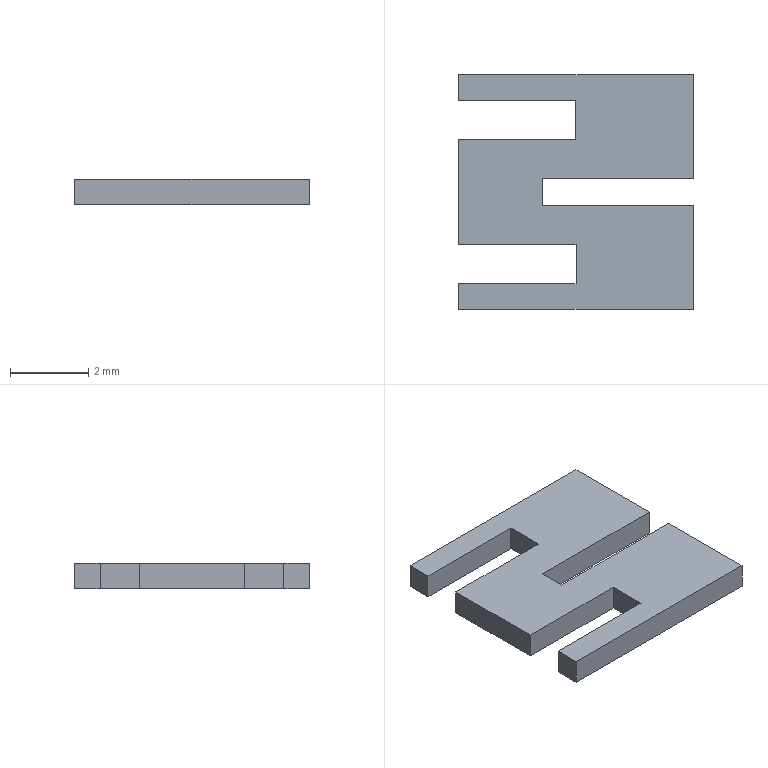Part | STEP file | RJ-USIO-V1_2-220411_176 | 1 solid | 18 faces | box 6 x 6 x 0.65 mm | volume 17.741 mm3 | plane 18
STEP:
#1=CARTESIAN_POINT('',(0.,0.,0.));
#2=DIRECTION('',(0.,0.,1.));
#3=DIRECTION('',(1.,0.,0.));
#4=AXIS2_PLACEMENT_3D('',#1,#2,#3);
#5=CARTESIAN_POINT('',(100.284,60.75,4.15));
#6=VERTEX_POINT('',#5);
#7=CARTESIAN_POINT('',(100.284,60.75,4.8));
#8=VERTEX_POINT('',#7);
#9=CARTESIAN_POINT('',(100.284,60.75,4.15));
#10=DIRECTION('',(0.,0.,1.));
#11=VECTOR('',#10,1.);
#12=LINE('',#9,#11);
#13=CARTESIAN_POINT('',(100.284,60.4,4.475));
#14=DIRECTION('',(1.,0.000000012,0.));
#15=DIRECTION('',(0.,0.,1.));
#16=AXIS2_PLACEMENT_3D('',#13,#14,#15);
#17=PLANE('',#16);
#18=CARTESIAN_POINT('',(-0.325,-0.35));
#19=DIRECTION('',(1.,0.));
#20=VECTOR('',#19,1.);
#21=LINE('',#18,#20);
#22=(GEOMETRIC_REPRESENTATION_CONTEXT(2)PARAMETRIC_REPRESENTATION_CONTEXT()REPRESENTATION_CONTEXT('',''));
#23=DEFINITIONAL_REPRESENTATION('',(#21),#22);
#24=PCURVE('',#17,#23);
#25=CARTESIAN_POINT('',(102.217,60.75,4.475));
#26=DIRECTION('',(0.000000012,-1.,0.));
#27=DIRECTION('',(0.,0.,-1.));
#28=AXIS2_PLACEMENT_3D('',#25,#26,#27);
#29=PLANE('',#28);
#30=CARTESIAN_POINT('',(0.325,-1.933));
#31=DIRECTION('',(-1.,0.));
#32=VECTOR('',#31,1.);
#33=LINE('',#30,#32);
#34=(GEOMETRIC_REPRESENTATION_CONTEXT(2)PARAMETRIC_REPRESENTATION_CONTEXT()REPRESENTATION_CONTEXT('',''));
#35=DEFINITIONAL_REPRESENTATION('',(#33),#34);
#36=PCURVE('',#29,#35);
#37=SURFACE_CURVE('',#12,(#24,#36),.PCURVE_S1.);
#38=EDGE_CURVE('',#6,#8,#37,.T.);
#39=ORIENTED_EDGE('',*,*,#38,.F.);
#40=CARTESIAN_POINT('',(100.284,60.05,4.15));
#41=VERTEX_POINT('',#40);
#42=CARTESIAN_POINT('',(100.284,60.05,4.15));
#43=DIRECTION('',(-0.000000012,1.,0.));
#44=VECTOR('',#43,1.);
#45=LINE('',#42,#44);
#46=CARTESIAN_POINT('',(-0.325,0.35));
#47=DIRECTION('',(0.,-1.));
#48=VECTOR('',#47,1.);
#49=LINE('',#46,#48);
#50=(GEOMETRIC_REPRESENTATION_CONTEXT(2)PARAMETRIC_REPRESENTATION_CONTEXT()REPRESENTATION_CONTEXT('',''));
#51=DEFINITIONAL_REPRESENTATION('',(#49),#50);
#52=PCURVE('',#17,#51);
#53=CARTESIAN_POINT('',(101.15,60.4,4.15));
#54=DIRECTION('',(0.,0.,1.));
#55=DIRECTION('',(-0.000000012,1.,0.));
#56=AXIS2_PLACEMENT_3D('',#53,#54,#55);
#57=PLANE('',#56);
#58=CARTESIAN_POINT('',(-0.35,0.8663));
#59=DIRECTION('',(1.,0.));
#60=VECTOR('',#59,1.);
#61=LINE('',#58,#60);
#62=(GEOMETRIC_REPRESENTATION_CONTEXT(2)PARAMETRIC_REPRESENTATION_CONTEXT()REPRESENTATION_CONTEXT('',''));
#63=DEFINITIONAL_REPRESENTATION('',(#61),#62);
#64=PCURVE('',#57,#63);
#65=SURFACE_CURVE('',#45,(#52,#64),.PCURVE_S1.);
#66=EDGE_CURVE('',#41,#6,#65,.T.);
#67=ORIENTED_EDGE('',*,*,#66,.F.);
#68=CARTESIAN_POINT('',(100.284,60.05,4.8));
#69=VERTEX_POINT('',#68);
#70=CARTESIAN_POINT('',(100.284,60.05,4.15));
#71=DIRECTION('',(0.,0.,1.));
#72=VECTOR('',#71,1.);
#73=LINE('',#70,#72);
#74=CARTESIAN_POINT('',(-0.325,0.35));
#75=DIRECTION('',(1.,0.));
#76=VECTOR('',#75,1.);
#77=LINE('',#74,#76);
#78=(GEOMETRIC_REPRESENTATION_CONTEXT(2)PARAMETRIC_REPRESENTATION_CONTEXT()REPRESENTATION_CONTEXT('',''));
#79=DEFINITIONAL_REPRESENTATION('',(#77),#78);
#80=PCURVE('',#17,#79);
#81=CARTESIAN_POINT('',(102.217,60.05,4.475));
#82=DIRECTION('',(0.000000012,-1.,0.));
#83=DIRECTION('',(-1.,-0.000000012,0.));
#84=AXIS2_PLACEMENT_3D('',#81,#82,#83);
#85=PLANE('',#84);
#86=CARTESIAN_POINT('',(1.933,0.325));
#87=DIRECTION('',(0.,-1.));
#88=VECTOR('',#87,1.);
#89=LINE('',#86,#88);
#90=(GEOMETRIC_REPRESENTATION_CONTEXT(2)PARAMETRIC_REPRESENTATION_CONTEXT()REPRESENTATION_CONTEXT('',''));
#91=DEFINITIONAL_REPRESENTATION('',(#89),#90);
#92=PCURVE('',#85,#91);
#93=SURFACE_CURVE('',#73,(#80,#92),.PCURVE_S1.);
#94=EDGE_CURVE('',#41,#69,#93,.T.);
#95=ORIENTED_EDGE('',*,*,#94,.T.);
#96=CARTESIAN_POINT('',(100.284,60.05,4.8));
#97=DIRECTION('',(-0.000000012,1.,0.));
#98=VECTOR('',#97,1.);
#99=LINE('',#96,#98);
#100=CARTESIAN_POINT('',(0.325,0.35));
#101=DIRECTION('',(0.,-1.));
#102=VECTOR('',#101,1.);
#103=LINE('',#100,#102);
#104=(GEOMETRIC_REPRESENTATION_CONTEXT(2)PARAMETRIC_REPRESENTATION_CONTEXT()REPRESENTATION_CONTEXT('',''));
#105=DEFINITIONAL_REPRESENTATION('',(#103),#104);
#106=PCURVE('',#17,#105);
#107=CARTESIAN_POINT('',(101.15,60.4,4.8));
#108=DIRECTION('',(0.,0.,1.));
#109=DIRECTION('',(-0.000000012,1.,0.));
#110=AXIS2_PLACEMENT_3D('',#107,#108,#109);
#111=PLANE('',#110);
#112=CARTESIAN_POINT('',(-0.35,0.8663));
#113=DIRECTION('',(1.,0.));
#114=VECTOR('',#113,1.);
#115=LINE('',#112,#114);
#116=(GEOMETRIC_REPRESENTATION_CONTEXT(2)PARAMETRIC_REPRESENTATION_CONTEXT()REPRESENTATION_CONTEXT('',''));
#117=DEFINITIONAL_REPRESENTATION('',(#115),#116);
#118=PCURVE('',#111,#117);
#119=SURFACE_CURVE('',#99,(#106,#118),.PCURVE_S1.);
#120=EDGE_CURVE('',#69,#8,#119,.T.);
#121=ORIENTED_EDGE('',*,*,#120,.T.);
#122=EDGE_LOOP('',(#39,#67,#95,#121));
#123=FACE_BOUND('',#122,.F.);
#124=ADVANCED_FACE('',(#123),#17,.T.);
#125=CARTESIAN_POINT('',(104.15,60.75,4.15));
#126=VERTEX_POINT('',#125);
#127=CARTESIAN_POINT('',(104.15,60.75,4.8));
#128=VERTEX_POINT('',#127);
#129=CARTESIAN_POINT('',(104.15,60.75,4.15));
#130=DIRECTION('',(0.,0.,1.));
#131=VECTOR('',#130,1.);
#132=LINE('',#129,#131);
#133=CARTESIAN_POINT('',(0.325,1.933));
#134=DIRECTION('',(-1.,0.));
#135=VECTOR('',#134,1.);
#136=LINE('',#133,#135);
#137=(GEOMETRIC_REPRESENTATION_CONTEXT(2)PARAMETRIC_REPRESENTATION_CONTEXT()REPRESENTATION_CONTEXT('',''));
#138=DEFINITIONAL_REPRESENTATION('',(#136),#137);
#139=PCURVE('',#29,#138);
#140=CARTESIAN_POINT('',(104.15,62.075,4.475));
#141=DIRECTION('',(1.,0.000000012,0.));
#142=DIRECTION('',(0.,0.,1.));
#143=AXIS2_PLACEMENT_3D('',#140,#141,#142);
#144=PLANE('',#143);
#145=CARTESIAN_POINT('',(-0.325,1.325));
#146=DIRECTION('',(1.,0.));
#147=VECTOR('',#146,1.);
#148=LINE('',#145,#147);
#149=(GEOMETRIC_REPRESENTATION_CONTEXT(2)PARAMETRIC_REPRESENTATION_CONTEXT()REPRESENTATION_CONTEXT('',''));
#150=DEFINITIONAL_REPRESENTATION('',(#148),#149);
#151=PCURVE('',#144,#150);
#152=SURFACE_CURVE('',#132,(#139,#151),.PCURVE_S1.);
#153=EDGE_CURVE('',#126,#128,#152,.T.);
#154=ORIENTED_EDGE('',*,*,#153,.F.);
#155=CARTESIAN_POINT('',(100.284,60.75,4.15));
#156=DIRECTION('',(1.,0.000000012,0.));
#157=VECTOR('',#156,1.);
#158=LINE('',#155,#157);
#159=CARTESIAN_POINT('',(0.325,-1.933));
#160=DIRECTION('',(0.,1.));
#161=VECTOR('',#160,1.);
#162=LINE('',#159,#161);
#163=(GEOMETRIC_REPRESENTATION_CONTEXT(2)PARAMETRIC_REPRESENTATION_CONTEXT()REPRESENTATION_CONTEXT('',''));
#164=DEFINITIONAL_REPRESENTATION('',(#162),#163);
#165=PCURVE('',#29,#164);
#166=CARTESIAN_POINT('',(0.35,0.8663));
#167=DIRECTION('',(0.,-1.));
#168=VECTOR('',#167,1.);
#169=LINE('',#166,#168);
#170=(GEOMETRIC_REPRESENTATION_CONTEXT(2)PARAMETRIC_REPRESENTATION_CONTEXT()REPRESENTATION_CONTEXT('',''));
#171=DEFINITIONAL_REPRESENTATION('',(#169),#170);
#172=PCURVE('',#57,#171);
#173=SURFACE_CURVE('',#158,(#165,#172),.PCURVE_S1.);
#174=EDGE_CURVE('',#6,#126,#173,.T.);
#175=ORIENTED_EDGE('',*,*,#174,.F.);
#176=ORIENTED_EDGE('',*,*,#38,.T.);
#177=CARTESIAN_POINT('',(100.284,60.75,4.8));
#178=DIRECTION('',(1.,0.000000012,0.));
#179=VECTOR('',#178,1.);
#180=LINE('',#177,#179);
#181=CARTESIAN_POINT('',(-0.325,-1.933));
#182=DIRECTION('',(0.,1.));
#183=VECTOR('',#182,1.);
#184=LINE('',#181,#183);
#185=(GEOMETRIC_REPRESENTATION_CONTEXT(2)PARAMETRIC_REPRESENTATION_CONTEXT()REPRESENTATION_CONTEXT('',''));
#186=DEFINITIONAL_REPRESENTATION('',(#184),#185);
#187=PCURVE('',#29,#186);
#188=CARTESIAN_POINT('',(0.35,0.8663));
#189=DIRECTION('',(0.,-1.));
#190=VECTOR('',#189,1.);
#191=LINE('',#188,#190);
#192=(GEOMETRIC_REPRESENTATION_CONTEXT(2)PARAMETRIC_REPRESENTATION_CONTEXT()REPRESENTATION_CONTEXT('',''));
#193=DEFINITIONAL_REPRESENTATION('',(#191),#192);
#194=PCURVE('',#111,#193);
#195=SURFACE_CURVE('',#180,(#187,#194),.PCURVE_S1.);
#196=EDGE_CURVE('',#8,#128,#195,.T.);
#197=ORIENTED_EDGE('',*,*,#196,.T.);
#198=EDGE_LOOP('',(#154,#175,#176,#197));
#199=FACE_BOUND('',#198,.F.);
#200=ADVANCED_FACE('',(#199),#29,.T.);
#201=CARTESIAN_POINT('',(104.15,63.4,4.15));
#202=VERTEX_POINT('',#201);
#203=CARTESIAN_POINT('',(104.15,63.4,4.8));
#204=VERTEX_POINT('',#203);
#205=CARTESIAN_POINT('',(104.15,63.4,4.15));
#206=DIRECTION('',(0.,0.,1.));
#207=VECTOR('',#206,1.);
#208=LINE('',#205,#207);
#209=CARTESIAN_POINT('',(-0.325,-1.325));
#210=DIRECTION('',(1.,0.));
#211=VECTOR('',#210,1.);
#212=LINE('',#209,#211);
#213=(GEOMETRIC_REPRESENTATION_CONTEXT(2)PARAMETRIC_REPRESENTATION_CONTEXT()REPRESENTATION_CONTEXT('',''));
#214=DEFINITIONAL_REPRESENTATION('',(#212),#213);
#215=PCURVE('',#144,#214);
#216=CARTESIAN_POINT('',(101.15,63.4,4.475));
#217=DIRECTION('',(0.000000012,-1.,0.));
#218=DIRECTION('',(0.,0.,1.));
#219=AXIS2_PLACEMENT_3D('',#216,#217,#218);
#220=PLANE('',#219);
#221=CARTESIAN_POINT('',(-0.325,-3.));
#222=DIRECTION('',(1.,0.));
#223=VECTOR('',#222,1.);
#224=LINE('',#221,#223);
#225=(GEOMETRIC_REPRESENTATION_CONTEXT(2)PARAMETRIC_REPRESENTATION_CONTEXT()REPRESENTATION_CONTEXT('',''));
#226=DEFINITIONAL_REPRESENTATION('',(#224),#225);
#227=PCURVE('',#220,#226);
#228=SURFACE_CURVE('',#208,(#215,#227),.PCURVE_S1.);
#229=EDGE_CURVE('',#202,#204,#228,.T.);
#230=ORIENTED_EDGE('',*,*,#229,.F.);
#231=CARTESIAN_POINT('',(104.15,60.75,4.15));
#232=DIRECTION('',(-0.000000012,1.,0.));
#233=VECTOR('',#232,1.);
#234=LINE('',#231,#233);
#235=CARTESIAN_POINT('',(-0.325,1.325));
#236=DIRECTION('',(0.,-1.));
#237=VECTOR('',#236,1.);
#238=LINE('',#235,#237);
#239=(GEOMETRIC_REPRESENTATION_CONTEXT(2)PARAMETRIC_REPRESENTATION_CONTEXT()REPRESENTATION_CONTEXT('',''));
#240=DEFINITIONAL_REPRESENTATION('',(#238),#239);
#241=PCURVE('',#144,#240);
#242=CARTESIAN_POINT('',(0.35,-3.));
#243=DIRECTION('',(1.,0.));
#244=VECTOR('',#243,1.);
#245=LINE('',#242,#244);
#246=(GEOMETRIC_REPRESENTATION_CONTEXT(2)PARAMETRIC_REPRESENTATION_CONTEXT()REPRESENTATION_CONTEXT('',''));
#247=DEFINITIONAL_REPRESENTATION('',(#245),#246);
#248=PCURVE('',#57,#247);
#249=SURFACE_CURVE('',#234,(#241,#248),.PCURVE_S1.);
#250=EDGE_CURVE('',#126,#202,#249,.T.);
#251=ORIENTED_EDGE('',*,*,#250,.F.);
#252=ORIENTED_EDGE('',*,*,#153,.T.);
#253=CARTESIAN_POINT('',(104.15,60.75,4.8));
#254=DIRECTION('',(-0.000000012,1.,0.));
#255=VECTOR('',#254,1.);
#256=LINE('',#253,#255);
#257=CARTESIAN_POINT('',(0.325,1.325));
#258=DIRECTION('',(0.,-1.));
#259=VECTOR('',#258,1.);
#260=LINE('',#257,#259);
#261=(GEOMETRIC_REPRESENTATION_CONTEXT(2)PARAMETRIC_REPRESENTATION_CONTEXT()REPRESENTATION_CONTEXT('',''));
#262=DEFINITIONAL_REPRESENTATION('',(#260),#261);
#263=PCURVE('',#144,#262);
#264=CARTESIAN_POINT('',(0.35,-3.));
#265=DIRECTION('',(1.,0.));
#266=VECTOR('',#265,1.);
#267=LINE('',#264,#266);
#268=(GEOMETRIC_REPRESENTATION_CONTEXT(2)PARAMETRIC_REPRESENTATION_CONTEXT()REPRESENTATION_CONTEXT('',''));
#269=DEFINITIONAL_REPRESENTATION('',(#267),#268);
#270=PCURVE('',#111,#269);
#271=SURFACE_CURVE('',#256,(#263,#270),.PCURVE_S1.);
#272=EDGE_CURVE('',#128,#204,#271,.T.);
#273=ORIENTED_EDGE('',*,*,#272,.T.);
#274=EDGE_LOOP('',(#230,#251,#252,#273));
#275=FACE_BOUND('',#274,.F.);
#276=ADVANCED_FACE('',(#275),#144,.T.);
#277=CARTESIAN_POINT('',(98.15,63.4,4.8));
#278=VERTEX_POINT('',#277);
#279=CARTESIAN_POINT('',(98.15,63.4,4.15));
#280=VERTEX_POINT('',#279);
#281=CARTESIAN_POINT('',(98.15,63.4,4.8));
#282=DIRECTION('',(0.,0.,-1.));
#283=VECTOR('',#282,1.);
#284=LINE('',#281,#283);
#285=CARTESIAN_POINT('',(0.325,3.));
#286=DIRECTION('',(-1.,0.));
#287=VECTOR('',#286,1.);
#288=LINE('',#285,#287);
#289=(GEOMETRIC_REPRESENTATION_CONTEXT(2)PARAMETRIC_REPRESENTATION_CONTEXT()REPRESENTATION_CONTEXT('',''));
#290=DEFINITIONAL_REPRESENTATION('',(#288),#289);
#291=PCURVE('',#220,#290);
#292=CARTESIAN_POINT('',(98.15,63.075,4.475));
#293=DIRECTION('',(1.,0.000000012,0.));
#294=DIRECTION('',(0.,0.,-1.));
#295=AXIS2_PLACEMENT_3D('',#292,#293,#294);
#296=PLANE('',#295);
#297=CARTESIAN_POINT('',(-0.325,0.325));
#298=DIRECTION('',(1.,0.));
#299=VECTOR('',#298,1.);
#300=LINE('',#297,#299);
#301=(GEOMETRIC_REPRESENTATION_CONTEXT(2)PARAMETRIC_REPRESENTATION_CONTEXT()REPRESENTATION_CONTEXT('',''));
#302=DEFINITIONAL_REPRESENTATION('',(#300),#301);
#303=PCURVE('',#296,#302);
#304=SURFACE_CURVE('',#284,(#291,#303),.PCURVE_S1.);
#305=EDGE_CURVE('',#278,#280,#304,.T.);
#306=ORIENTED_EDGE('',*,*,#305,.T.);
#307=CARTESIAN_POINT('',(104.15,63.4,4.15));
#308=DIRECTION('',(-1.,-0.000000012,0.));
#309=VECTOR('',#308,1.);
#310=LINE('',#307,#309);
#311=CARTESIAN_POINT('',(-0.325,-3.));
#312=DIRECTION('',(0.,1.));
#313=VECTOR('',#312,1.);
#314=LINE('',#311,#313);
#315=(GEOMETRIC_REPRESENTATION_CONTEXT(2)PARAMETRIC_REPRESENTATION_CONTEXT()REPRESENTATION_CONTEXT('',''));
#316=DEFINITIONAL_REPRESENTATION('',(#314),#315);
#317=PCURVE('',#220,#316);
#318=CARTESIAN_POINT('',(3.,-3.));
#319=DIRECTION('',(0.,1.));
#320=VECTOR('',#319,1.);
#321=LINE('',#318,#320);
#322=(GEOMETRIC_REPRESENTATION_CONTEXT(2)PARAMETRIC_REPRESENTATION_CONTEXT()REPRESENTATION_CONTEXT('',''));
#323=DEFINITIONAL_REPRESENTATION('',(#321),#322);
#324=PCURVE('',#57,#323);
#325=SURFACE_CURVE('',#310,(#317,#324),.PCURVE_S1.);
#326=EDGE_CURVE('',#202,#280,#325,.T.);
#327=ORIENTED_EDGE('',*,*,#326,.F.);
#328=ORIENTED_EDGE('',*,*,#229,.T.);
#329=CARTESIAN_POINT('',(104.15,63.4,4.8));
#330=DIRECTION('',(-1.,-0.000000012,0.));
#331=VECTOR('',#330,1.);
#332=LINE('',#329,#331);
#333=CARTESIAN_POINT('',(0.325,-3.));
#334=DIRECTION('',(0.,1.));
#335=VECTOR('',#334,1.);
#336=LINE('',#333,#335);
#337=(GEOMETRIC_REPRESENTATION_CONTEXT(2)PARAMETRIC_REPRESENTATION_CONTEXT()REPRESENTATION_CONTEXT('',''));
#338=DEFINITIONAL_REPRESENTATION('',(#336),#337);
#339=PCURVE('',#220,#338);
#340=CARTESIAN_POINT('',(3.,-3.));
#341=DIRECTION('',(0.,1.));
#342=VECTOR('',#341,1.);
#343=LINE('',#340,#342);
#344=(GEOMETRIC_REPRESENTATION_CONTEXT(2)PARAMETRIC_REPRESENTATION_CONTEXT()REPRESENTATION_CONTEXT('',''));
#345=DEFINITIONAL_REPRESENTATION('',(#343),#344);
#346=PCURVE('',#111,#345);
#347=SURFACE_CURVE('',#332,(#339,#346),.PCURVE_S1.);
#348=EDGE_CURVE('',#204,#278,#347,.T.);
#349=ORIENTED_EDGE('',*,*,#348,.T.);
#350=EDGE_LOOP('',(#306,#327,#328,#349));
#351=FACE_BOUND('',#350,.F.);
#352=ADVANCED_FACE('',(#351),#220,.F.);
#353=CARTESIAN_POINT('',(98.15,62.75,4.15));
#354=VERTEX_POINT('',#353);
#355=CARTESIAN_POINT('',(98.15,62.75,4.8));
#356=VERTEX_POINT('',#355);
#357=CARTESIAN_POINT('',(98.15,62.75,4.15));
#358=DIRECTION('',(0.,0.,1.));
#359=VECTOR('',#358,1.);
#360=LINE('',#357,#359);
#361=CARTESIAN_POINT('',(0.325,-0.325));
#362=DIRECTION('',(-1.,0.));
#363=VECTOR('',#362,1.);
#364=LINE('',#361,#363);
#365=(GEOMETRIC_REPRESENTATION_CONTEXT(2)PARAMETRIC_REPRESENTATION_CONTEXT()REPRESENTATION_CONTEXT('',''));
#366=DEFINITIONAL_REPRESENTATION('',(#364),#365);
#367=PCURVE('',#296,#366);
#368=CARTESIAN_POINT('',(99.65,62.75,4.475));
#369=DIRECTION('',(0.000000012,-1.,0.));
#370=DIRECTION('',(0.,0.,-1.));
#371=AXIS2_PLACEMENT_3D('',#368,#369,#370);
#372=PLANE('',#371);
#373=CARTESIAN_POINT('',(0.325,-1.5));
#374=DIRECTION('',(-1.,0.));
#375=VECTOR('',#374,1.);
#376=LINE('',#373,#375);
#377=(GEOMETRIC_REPRESENTATION_CONTEXT(2)PARAMETRIC_REPRESENTATION_CONTEXT()REPRESENTATION_CONTEXT('',''));
#378=DEFINITIONAL_REPRESENTATION('',(#376),#377);
#379=PCURVE('',#372,#378);
#380=SURFACE_CURVE('',#360,(#367,#379),.PCURVE_S1.);
#381=EDGE_CURVE('',#354,#356,#380,.T.);
#382=ORIENTED_EDGE('',*,*,#381,.F.);
#383=CARTESIAN_POINT('',(98.15,63.4,4.15));
#384=DIRECTION('',(0.000000012,-1.,0.));
#385=VECTOR('',#384,1.);
#386=LINE('',#383,#385);
#387=CARTESIAN_POINT('',(0.325,0.325));
#388=DIRECTION('',(0.,-1.));
#389=VECTOR('',#388,1.);
#390=LINE('',#387,#389);
#391=(GEOMETRIC_REPRESENTATION_CONTEXT(2)PARAMETRIC_REPRESENTATION_CONTEXT()REPRESENTATION_CONTEXT('',''));
#392=DEFINITIONAL_REPRESENTATION('',(#390),#391);
#393=PCURVE('',#296,#392);
#394=CARTESIAN_POINT('',(3.,3.));
#395=DIRECTION('',(-1.,0.));
#396=VECTOR('',#395,1.);
#397=LINE('',#394,#396);
#398=(GEOMETRIC_REPRESENTATION_CONTEXT(2)PARAMETRIC_REPRESENTATION_CONTEXT()REPRESENTATION_CONTEXT('',''));
#399=DEFINITIONAL_REPRESENTATION('',(#397),#398);
#400=PCURVE('',#57,#399);
#401=SURFACE_CURVE('',#386,(#393,#400),.PCURVE_S1.);
#402=EDGE_CURVE('',#280,#354,#401,.T.);
#403=ORIENTED_EDGE('',*,*,#402,.F.);
#404=ORIENTED_EDGE('',*,*,#305,.F.);
#405=CARTESIAN_POINT('',(98.15,63.4,4.8));
#406=DIRECTION('',(0.000000012,-1.,0.));
#407=VECTOR('',#406,1.);
#408=LINE('',#405,#407);
#409=CARTESIAN_POINT('',(-0.325,0.325));
#410=DIRECTION('',(0.,-1.));
#411=VECTOR('',#410,1.);
#412=LINE('',#409,#411);
#413=(GEOMETRIC_REPRESENTATION_CONTEXT(2)PARAMETRIC_REPRESENTATION_CONTEXT()REPRESENTATION_CONTEXT('',''));
#414=DEFINITIONAL_REPRESENTATION('',(#412),#413);
#415=PCURVE('',#296,#414);
#416=CARTESIAN_POINT('',(3.,3.));
#417=DIRECTION('',(-1.,0.));
#418=VECTOR('',#417,1.);
#419=LINE('',#416,#418);
#420=(GEOMETRIC_REPRESENTATION_CONTEXT(2)PARAMETRIC_REPRESENTATION_CONTEXT()REPRESENTATION_CONTEXT('',''));
#421=DEFINITIONAL_REPRESENTATION('',(#419),#420);
#422=PCURVE('',#111,#421);
#423=SURFACE_CURVE('',#408,(#415,#422),.PCURVE_S1.);
#424=EDGE_CURVE('',#278,#356,#423,.T.);
#425=ORIENTED_EDGE('',*,*,#424,.T.);
#426=EDGE_LOOP('',(#382,#403,#404,#425));
#427=FACE_BOUND('',#426,.F.);
#428=ADVANCED_FACE('',(#427),#296,.F.);
#429=CARTESIAN_POINT('',(101.15,62.75,4.15));
#430=VERTEX_POINT('',#429);
#431=CARTESIAN_POINT('',(101.15,62.75,4.8));
#432=VERTEX_POINT('',#431);
#433=CARTESIAN_POINT('',(101.15,62.75,4.15));
#434=DIRECTION('',(0.,0.,1.));
#435=VECTOR('',#434,1.);
#436=LINE('',#433,#435);
#437=CARTESIAN_POINT('',(0.325,1.5));
#438=DIRECTION('',(-1.,0.));
#439=VECTOR('',#438,1.);
#440=LINE('',#437,#439);
#441=(GEOMETRIC_REPRESENTATION_CONTEXT(2)PARAMETRIC_REPRESENTATION_CONTEXT()REPRESENTATION_CONTEXT('',''));
#442=DEFINITIONAL_REPRESENTATION('',(#440),#441);
#443=PCURVE('',#372,#442);
#444=CARTESIAN_POINT('',(101.15,62.25,4.475));
#445=DIRECTION('',(1.,0.000000012,0.));
#446=DIRECTION('',(0.,0.,-1.));
#447=AXIS2_PLACEMENT_3D('',#444,#445,#446);
#448=PLANE('',#447);
#449=CARTESIAN_POINT('',(0.325,0.5));
#450=DIRECTION('',(-1.,0.));
#451=VECTOR('',#450,1.);
#452=LINE('',#449,#451);
#453=(GEOMETRIC_REPRESENTATION_CONTEXT(2)PARAMETRIC_REPRESENTATION_CONTEXT()REPRESENTATION_CONTEXT('',''));
#454=DEFINITIONAL_REPRESENTATION('',(#452),#453);
#455=PCURVE('',#448,#454);
#456=SURFACE_CURVE('',#436,(#443,#455),.PCURVE_S1.);
#457=EDGE_CURVE('',#430,#432,#456,.T.);
#458=ORIENTED_EDGE('',*,*,#457,.F.);
#459=CARTESIAN_POINT('',(98.15,62.75,4.15));
#460=DIRECTION('',(1.,0.000000012,0.));
#461=VECTOR('',#460,1.);
#462=LINE('',#459,#461);
#463=CARTESIAN_POINT('',(0.325,-1.5));
#464=DIRECTION('',(0.,1.));
#465=VECTOR('',#464,1.);
#466=LINE('',#463,#465);
#467=(GEOMETRIC_REPRESENTATION_CONTEXT(2)PARAMETRIC_REPRESENTATION_CONTEXT()REPRESENTATION_CONTEXT('',''));
#468=DEFINITIONAL_REPRESENTATION('',(#466),#467);
#469=PCURVE('',#372,#468);
#470=CARTESIAN_POINT('',(2.35,3.));
#471=DIRECTION('',(0.,-1.));
#472=VECTOR('',#471,1.);
#473=LINE('',#470,#472);
#474=(GEOMETRIC_REPRESENTATION_CONTEXT(2)PARAMETRIC_REPRESENTATION_CONTEXT()REPRESENTATION_CONTEXT('',''));
#475=DEFINITIONAL_REPRESENTATION('',(#473),#474);
#476=PCURVE('',#57,#475);
#477=SURFACE_CURVE('',#462,(#469,#476),.PCURVE_S1.);
#478=EDGE_CURVE('',#354,#430,#477,.T.);
#479=ORIENTED_EDGE('',*,*,#478,.F.);
#480=ORIENTED_EDGE('',*,*,#381,.T.);
#481=CARTESIAN_POINT('',(98.15,62.75,4.8));
#482=DIRECTION('',(1.,0.000000012,0.));
#483=VECTOR('',#482,1.);
#484=LINE('',#481,#483);
#485=CARTESIAN_POINT('',(-0.325,-1.5));
#486=DIRECTION('',(0.,1.));
#487=VECTOR('',#486,1.);
#488=LINE('',#485,#487);
#489=(GEOMETRIC_REPRESENTATION_CONTEXT(2)PARAMETRIC_REPRESENTATION_CONTEXT()REPRESENTATION_CONTEXT('',''));
#490=DEFINITIONAL_REPRESENTATION('',(#488),#489);
#491=PCURVE('',#372,#490);
#492=CARTESIAN_POINT('',(2.35,3.));
#493=DIRECTION('',(0.,-1.));
#494=VECTOR('',#493,1.);
#495=LINE('',#492,#494);
#496=(GEOMETRIC_REPRESENTATION_CONTEXT(2)PARAMETRIC_REPRESENTATION_CONTEXT()REPRESENTATION_CONTEXT('',''));
#497=DEFINITIONAL_REPRESENTATION('',(#495),#496);
#498=PCURVE('',#111,#497);
#499=SURFACE_CURVE('',#484,(#491,#498),.PCURVE_S1.);
#500=EDGE_CURVE('',#356,#432,#499,.T.);
#501=ORIENTED_EDGE('',*,*,#500,.T.);
#502=EDGE_LOOP('',(#458,#479,#480,#501));
#503=FACE_BOUND('',#502,.F.);
#504=ADVANCED_FACE('',(#503),#372,.T.);
#505=CARTESIAN_POINT('',(101.15,61.75,4.15));
#506=VERTEX_POINT('',#505);
#507=CARTESIAN_POINT('',(101.15,61.75,4.8));
#508=VERTEX_POINT('',#507);
#509=CARTESIAN_POINT('',(101.15,61.75,4.15));
#510=DIRECTION('',(0.,0.,1.));
#511=VECTOR('',#510,1.);
#512=LINE('',#509,#511);
#513=CARTESIAN_POINT('',(0.325,-0.5));
#514=DIRECTION('',(-1.,0.));
#515=VECTOR('',#514,1.);
#516=LINE('',#513,#515);
#517=(GEOMETRIC_REPRESENTATION_CONTEXT(2)PARAMETRIC_REPRESENTATION_CONTEXT()REPRESENTATION_CONTEXT('',''));
#518=DEFINITIONAL_REPRESENTATION('',(#516),#517);
#519=PCURVE('',#448,#518);
#520=CARTESIAN_POINT('',(99.65,61.75,4.475));
#521=DIRECTION('',(0.000000012,-1.,0.));
#522=DIRECTION('',(-1.,-0.000000012,0.));
#523=AXIS2_PLACEMENT_3D('',#520,#521,#522);
#524=PLANE('',#523);
#525=CARTESIAN_POINT('',(-1.5,0.325));
#526=DIRECTION('',(0.,-1.));
#527=VECTOR('',#526,1.);
#528=LINE('',#525,#527);
#529=(GEOMETRIC_REPRESENTATION_CONTEXT(2)PARAMETRIC_REPRESENTATION_CONTEXT()REPRESENTATION_CONTEXT('',''));
#530=DEFINITIONAL_REPRESENTATION('',(#528),#529);
#531=PCURVE('',#524,#530);
#532=SURFACE_CURVE('',#512,(#519,#531),.PCURVE_S1.);
#533=EDGE_CURVE('',#506,#508,#532,.T.);
#534=ORIENTED_EDGE('',*,*,#533,.F.);
#535=CARTESIAN_POINT('',(101.15,62.75,4.15));
#536=DIRECTION('',(0.000000012,-1.,0.));
#537=VECTOR('',#536,1.);
#538=LINE('',#535,#537);
#539=CARTESIAN_POINT('',(0.325,0.5));
#540=DIRECTION('',(0.,-1.));
#541=VECTOR('',#540,1.);
#542=LINE('',#539,#541);
#543=(GEOMETRIC_REPRESENTATION_CONTEXT(2)PARAMETRIC_REPRESENTATION_CONTEXT()REPRESENTATION_CONTEXT('',''));
#544=DEFINITIONAL_REPRESENTATION('',(#542),#543);
#545=PCURVE('',#448,#544);
#546=CARTESIAN_POINT('',(2.35,0.));
#547=DIRECTION('',(-1.,0.));
#548=VECTOR('',#547,1.);
#549=LINE('',#546,#548);
#550=(GEOMETRIC_REPRESENTATION_CONTEXT(2)PARAMETRIC_REPRESENTATION_CONTEXT()REPRESENTATION_CONTEXT('',''));
#551=DEFINITIONAL_REPRESENTATION('',(#549),#550);
#552=PCURVE('',#57,#551);
#553=SURFACE_CURVE('',#538,(#545,#552),.PCURVE_S1.);
#554=EDGE_CURVE('',#430,#506,#553,.T.);
#555=ORIENTED_EDGE('',*,*,#554,.F.);
#556=ORIENTED_EDGE('',*,*,#457,.T.);
#557=CARTESIAN_POINT('',(101.15,62.75,4.8));
#558=DIRECTION('',(0.000000012,-1.,0.));
#559=VECTOR('',#558,1.);
#560=LINE('',#557,#559);
#561=CARTESIAN_POINT('',(-0.325,0.5));
#562=DIRECTION('',(0.,-1.));
#563=VECTOR('',#562,1.);
#564=LINE('',#561,#563);
#565=(GEOMETRIC_REPRESENTATION_CONTEXT(2)PARAMETRIC_REPRESENTATION_CONTEXT()REPRESENTATION_CONTEXT('',''));
#566=DEFINITIONAL_REPRESENTATION('',(#564),#565);
#567=PCURVE('',#448,#566);
#568=CARTESIAN_POINT('',(2.35,0.));
#569=DIRECTION('',(-1.,0.));
#570=VECTOR('',#569,1.);
#571=LINE('',#568,#570);
#572=(GEOMETRIC_REPRESENTATION_CONTEXT(2)PARAMETRIC_REPRESENTATION_CONTEXT()REPRESENTATION_CONTEXT('',''));
#573=DEFINITIONAL_REPRESENTATION('',(#571),#572);
#574=PCURVE('',#111,#573);
#575=SURFACE_CURVE('',#560,(#567,#574),.PCURVE_S1.);
#576=EDGE_CURVE('',#432,#508,#575,.T.);
#577=ORIENTED_EDGE('',*,*,#576,.T.);
#578=EDGE_LOOP('',(#534,#555,#556,#577));
#579=FACE_BOUND('',#578,.F.);
#580=ADVANCED_FACE('',(#579),#448,.F.);
#581=CARTESIAN_POINT('',(98.15,61.75,4.15));
#582=VERTEX_POINT('',#581);
#583=CARTESIAN_POINT('',(98.15,61.75,4.8));
#584=VERTEX_POINT('',#583);
#585=CARTESIAN_POINT('',(98.15,61.75,4.15));
#586=DIRECTION('',(0.,0.,1.));
#587=VECTOR('',#586,1.);
#588=LINE('',#585,#587);
#589=CARTESIAN_POINT('',(1.5,0.325));
#590=DIRECTION('',(0.,-1.));
#591=VECTOR('',#590,1.);
#592=LINE('',#589,#591);
#593=(GEOMETRIC_REPRESENTATION_CONTEXT(2)PARAMETRIC_REPRESENTATION_CONTEXT()REPRESENTATION_CONTEXT('',''));
#594=DEFINITIONAL_REPRESENTATION('',(#592),#593);
#595=PCURVE('',#524,#594);
#596=CARTESIAN_POINT('',(98.15,60.4,4.475));
#597=DIRECTION('',(1.,0.000000012,0.));
#598=DIRECTION('',(0.,0.,-1.));
#599=AXIS2_PLACEMENT_3D('',#596,#597,#598);
#600=PLANE('',#599);
#601=CARTESIAN_POINT('',(0.325,1.35));
#602=DIRECTION('',(-1.,0.));
#603=VECTOR('',#602,1.);
#604=LINE('',#601,#603);
#605=(GEOMETRIC_REPRESENTATION_CONTEXT(2)PARAMETRIC_REPRESENTATION_CONTEXT()REPRESENTATION_CONTEXT('',''));
#606=DEFINITIONAL_REPRESENTATION('',(#604),#605);
#607=PCURVE('',#600,#606);
#608=SURFACE_CURVE('',#588,(#595,#607),.PCURVE_S1.);
#609=EDGE_CURVE('',#582,#584,#608,.T.);
#610=ORIENTED_EDGE('',*,*,#609,.F.);
#611=CARTESIAN_POINT('',(101.15,61.75,4.15));
#612=DIRECTION('',(-1.,-0.000000012,0.));
#613=VECTOR('',#612,1.);
#614=LINE('',#611,#613);
#615=CARTESIAN_POINT('',(-1.5,0.325));
#616=DIRECTION('',(1.,0.));
#617=VECTOR('',#616,1.);
#618=LINE('',#615,#617);
#619=(GEOMETRIC_REPRESENTATION_CONTEXT(2)PARAMETRIC_REPRESENTATION_CONTEXT()REPRESENTATION_CONTEXT('',''));
#620=DEFINITIONAL_REPRESENTATION('',(#618),#619);
#621=PCURVE('',#524,#620);
#622=CARTESIAN_POINT('',(1.35,0.));
#623=DIRECTION('',(0.,1.));
#624=VECTOR('',#623,1.);
#625=LINE('',#622,#624);
#626=(GEOMETRIC_REPRESENTATION_CONTEXT(2)PARAMETRIC_REPRESENTATION_CONTEXT()REPRESENTATION_CONTEXT('',''));
#627=DEFINITIONAL_REPRESENTATION('',(#625),#626);
#628=PCURVE('',#57,#627);
#629=SURFACE_CURVE('',#614,(#621,#628),.PCURVE_S1.);
#630=EDGE_CURVE('',#506,#582,#629,.T.);
#631=ORIENTED_EDGE('',*,*,#630,.F.);
#632=ORIENTED_EDGE('',*,*,#533,.T.);
#633=CARTESIAN_POINT('',(101.15,61.75,4.8));
#634=DIRECTION('',(-1.,-0.000000012,0.));
#635=VECTOR('',#634,1.);
#636=LINE('',#633,#635);
#637=CARTESIAN_POINT('',(-1.5,-0.325));
#638=DIRECTION('',(1.,0.));
#639=VECTOR('',#638,1.);
#640=LINE('',#637,#639);
#641=(GEOMETRIC_REPRESENTATION_CONTEXT(2)PARAMETRIC_REPRESENTATION_CONTEXT()REPRESENTATION_CONTEXT('',''));
#642=DEFINITIONAL_REPRESENTATION('',(#640),#641);
#643=PCURVE('',#524,#642);
#644=CARTESIAN_POINT('',(1.35,0.));
#645=DIRECTION('',(0.,1.));
#646=VECTOR('',#645,1.);
#647=LINE('',#644,#646);
#648=(GEOMETRIC_REPRESENTATION_CONTEXT(2)PARAMETRIC_REPRESENTATION_CONTEXT()REPRESENTATION_CONTEXT('',''));
#649=DEFINITIONAL_REPRESENTATION('',(#647),#648);
#650=PCURVE('',#111,#649);
#651=SURFACE_CURVE('',#636,(#643,#650),.PCURVE_S1.);
#652=EDGE_CURVE('',#508,#584,#651,.T.);
#653=ORIENTED_EDGE('',*,*,#652,.T.);
#654=EDGE_LOOP('',(#610,#631,#632,#653));
#655=FACE_BOUND('',#654,.F.);
#656=ADVANCED_FACE('',(#655),#524,.F.);
#657=CARTESIAN_POINT('',(98.15,59.05,4.15));
#658=VERTEX_POINT('',#657);
#659=CARTESIAN_POINT('',(98.15,59.05,4.8));
#660=VERTEX_POINT('',#659);
#661=CARTESIAN_POINT('',(98.15,59.05,4.15));
#662=DIRECTION('',(0.,0.,1.));
#663=VECTOR('',#662,1.);
#664=LINE('',#661,#663);
#665=CARTESIAN_POINT('',(0.325,-1.35));
#666=DIRECTION('',(-1.,0.));
#667=VECTOR('',#666,1.);
#668=LINE('',#665,#667);
#669=(GEOMETRIC_REPRESENTATION_CONTEXT(2)PARAMETRIC_REPRESENTATION_CONTEXT()REPRESENTATION_CONTEXT('',''));
#670=DEFINITIONAL_REPRESENTATION('',(#668),#669);
#671=PCURVE('',#600,#670);
#672=CARTESIAN_POINT('',(99.65,59.05,4.475));
#673=DIRECTION('',(0.000000012,-1.,0.));
#674=DIRECTION('',(0.,0.,-1.));
#675=AXIS2_PLACEMENT_3D('',#672,#673,#674);
#676=PLANE('',#675);
#677=CARTESIAN_POINT('',(0.325,-1.5));
#678=DIRECTION('',(-1.,0.));
#679=VECTOR('',#678,1.);
#680=LINE('',#677,#679);
#681=(GEOMETRIC_REPRESENTATION_CONTEXT(2)PARAMETRIC_REPRESENTATION_CONTEXT()REPRESENTATION_CONTEXT('',''));
#682=DEFINITIONAL_REPRESENTATION('',(#680),#681);
#683=PCURVE('',#676,#682);
#684=SURFACE_CURVE('',#664,(#671,#683),.PCURVE_S1.);
#685=EDGE_CURVE('',#658,#660,#684,.T.);
#686=ORIENTED_EDGE('',*,*,#685,.F.);
#687=CARTESIAN_POINT('',(98.15,61.75,4.15));
#688=DIRECTION('',(0.000000012,-1.,0.));
#689=VECTOR('',#688,1.);
#690=LINE('',#687,#689);
#691=CARTESIAN_POINT('',(0.325,1.35));
#692=DIRECTION('',(0.,-1.));
#693=VECTOR('',#692,1.);
#694=LINE('',#691,#693);
#695=(GEOMETRIC_REPRESENTATION_CONTEXT(2)PARAMETRIC_REPRESENTATION_CONTEXT()REPRESENTATION_CONTEXT('',''));
#696=DEFINITIONAL_REPRESENTATION('',(#694),#695);
#697=PCURVE('',#600,#696);
#698=CARTESIAN_POINT('',(1.35,3.));
#699=DIRECTION('',(-1.,0.));
#700=VECTOR('',#699,1.);
#701=LINE('',#698,#700);
#702=(GEOMETRIC_REPRESENTATION_CONTEXT(2)PARAMETRIC_REPRESENTATION_CONTEXT()REPRESENTATION_CONTEXT('',''));
#703=DEFINITIONAL_REPRESENTATION('',(#701),#702);
#704=PCURVE('',#57,#703);
#705=SURFACE_CURVE('',#690,(#697,#704),.PCURVE_S1.);
#706=EDGE_CURVE('',#582,#658,#705,.T.);
#707=ORIENTED_EDGE('',*,*,#706,.F.);
#708=ORIENTED_EDGE('',*,*,#609,.T.);
#709=CARTESIAN_POINT('',(98.15,61.75,4.8));
#710=DIRECTION('',(0.000000012,-1.,0.));
#711=VECTOR('',#710,1.);
#712=LINE('',#709,#711);
#713=CARTESIAN_POINT('',(-0.325,1.35));
#714=DIRECTION('',(0.,-1.));
#715=VECTOR('',#714,1.);
#716=LINE('',#713,#715);
#717=(GEOMETRIC_REPRESENTATION_CONTEXT(2)PARAMETRIC_REPRESENTATION_CONTEXT()REPRESENTATION_CONTEXT('',''));
#718=DEFINITIONAL_REPRESENTATION('',(#716),#717);
#719=PCURVE('',#600,#718);
#720=CARTESIAN_POINT('',(1.35,3.));
#721=DIRECTION('',(-1.,0.));
#722=VECTOR('',#721,1.);
#723=LINE('',#720,#722);
#724=(GEOMETRIC_REPRESENTATION_CONTEXT(2)PARAMETRIC_REPRESENTATION_CONTEXT()REPRESENTATION_CONTEXT('',''));
#725=DEFINITIONAL_REPRESENTATION('',(#723),#724);
#726=PCURVE('',#111,#725);
#727=SURFACE_CURVE('',#712,(#719,#726),.PCURVE_S1.);
#728=EDGE_CURVE('',#584,#660,#727,.T.);
#729=ORIENTED_EDGE('',*,*,#728,.T.);
#730=EDGE_LOOP('',(#686,#707,#708,#729));
#731=FACE_BOUND('',#730,.F.);
#732=ADVANCED_FACE('',(#731),#600,.F.);
#733=CARTESIAN_POINT('',(101.15,59.05,4.15));
#734=VERTEX_POINT('',#733);
#735=CARTESIAN_POINT('',(101.15,59.05,4.8));
#736=VERTEX_POINT('',#735);
#737=CARTESIAN_POINT('',(101.15,59.05,4.15));
#738=DIRECTION('',(0.,0.,1.));
#739=VECTOR('',#738,1.);
#740=LINE('',#737,#739);
#741=CARTESIAN_POINT('',(0.325,1.5));
#742=DIRECTION('',(-1.,0.));
#743=VECTOR('',#742,1.);
#744=LINE('',#741,#743);
#745=(GEOMETRIC_REPRESENTATION_CONTEXT(2)PARAMETRIC_REPRESENTATION_CONTEXT()REPRESENTATION_CONTEXT('',''));
#746=DEFINITIONAL_REPRESENTATION('',(#744),#745);
#747=PCURVE('',#676,#746);
#748=CARTESIAN_POINT('',(101.15,58.55,4.475));
#749=DIRECTION('',(1.,0.000000012,0.));
#750=DIRECTION('',(0.,0.,-1.));
#751=AXIS2_PLACEMENT_3D('',#748,#749,#750);
#752=PLANE('',#751);
#753=CARTESIAN_POINT('',(0.325,0.5));
#754=DIRECTION('',(-1.,0.));
#755=VECTOR('',#754,1.);
#756=LINE('',#753,#755);
#757=(GEOMETRIC_REPRESENTATION_CONTEXT(2)PARAMETRIC_REPRESENTATION_CONTEXT()REPRESENTATION_CONTEXT('',''));
#758=DEFINITIONAL_REPRESENTATION('',(#756),#757);
#759=PCURVE('',#752,#758);
#760=SURFACE_CURVE('',#740,(#747,#759),.PCURVE_S1.);
#761=EDGE_CURVE('',#734,#736,#760,.T.);
#762=ORIENTED_EDGE('',*,*,#761,.F.);
#763=CARTESIAN_POINT('',(98.15,59.05,4.15));
#764=DIRECTION('',(1.,0.000000012,0.));
#765=VECTOR('',#764,1.);
#766=LINE('',#763,#765);
#767=CARTESIAN_POINT('',(0.325,-1.5));
#768=DIRECTION('',(0.,1.));
#769=VECTOR('',#768,1.);
#770=LINE('',#767,#769);
#771=(GEOMETRIC_REPRESENTATION_CONTEXT(2)PARAMETRIC_REPRESENTATION_CONTEXT()REPRESENTATION_CONTEXT('',''));
#772=DEFINITIONAL_REPRESENTATION('',(#770),#771);
#773=PCURVE('',#676,#772);
#774=CARTESIAN_POINT('',(-1.35,3.));
#775=DIRECTION('',(0.,-1.));
#776=VECTOR('',#775,1.);
#777=LINE('',#774,#776);
#778=(GEOMETRIC_REPRESENTATION_CONTEXT(2)PARAMETRIC_REPRESENTATION_CONTEXT()REPRESENTATION_CONTEXT('',''));
#779=DEFINITIONAL_REPRESENTATION('',(#777),#778);
#780=PCURVE('',#57,#779);
#781=SURFACE_CURVE('',#766,(#773,#780),.PCURVE_S1.);
#782=EDGE_CURVE('',#658,#734,#781,.T.);
#783=ORIENTED_EDGE('',*,*,#782,.F.);
#784=ORIENTED_EDGE('',*,*,#685,.T.);
#785=CARTESIAN_POINT('',(98.15,59.05,4.8));
#786=DIRECTION('',(1.,0.000000012,0.));
#787=VECTOR('',#786,1.);
#788=LINE('',#785,#787);
#789=CARTESIAN_POINT('',(-0.325,-1.5));
#790=DIRECTION('',(0.,1.));
#791=VECTOR('',#790,1.);
#792=LINE('',#789,#791);
#793=(GEOMETRIC_REPRESENTATION_CONTEXT(2)PARAMETRIC_REPRESENTATION_CONTEXT()REPRESENTATION_CONTEXT('',''));
#794=DEFINITIONAL_REPRESENTATION('',(#792),#793);
#795=PCURVE('',#676,#794);
#796=CARTESIAN_POINT('',(-1.35,3.));
#797=DIRECTION('',(0.,-1.));
#798=VECTOR('',#797,1.);
#799=LINE('',#796,#798);
#800=(GEOMETRIC_REPRESENTATION_CONTEXT(2)PARAMETRIC_REPRESENTATION_CONTEXT()REPRESENTATION_CONTEXT('',''));
#801=DEFINITIONAL_REPRESENTATION('',(#799),#800);
#802=PCURVE('',#111,#801);
#803=SURFACE_CURVE('',#788,(#795,#802),.PCURVE_S1.);
#804=EDGE_CURVE('',#660,#736,#803,.T.);
#805=ORIENTED_EDGE('',*,*,#804,.T.);
#806=EDGE_LOOP('',(#762,#783,#784,#805));
#807=FACE_BOUND('',#806,.F.);
#808=ADVANCED_FACE('',(#807),#676,.T.);
#809=CARTESIAN_POINT('',(101.15,58.05,4.15));
#810=VERTEX_POINT('',#809);
#811=CARTESIAN_POINT('',(101.15,58.05,4.8));
#812=VERTEX_POINT('',#811);
#813=CARTESIAN_POINT('',(101.15,58.05,4.15));
#814=DIRECTION('',(0.,0.,1.));
#815=VECTOR('',#814,1.);
#816=LINE('',#813,#815);
#817=CARTESIAN_POINT('',(0.325,-0.5));
#818=DIRECTION('',(-1.,0.));
#819=VECTOR('',#818,1.);
#820=LINE('',#817,#819);
#821=(GEOMETRIC_REPRESENTATION_CONTEXT(2)PARAMETRIC_REPRESENTATION_CONTEXT()REPRESENTATION_CONTEXT('',''));
#822=DEFINITIONAL_REPRESENTATION('',(#820),#821);
#823=PCURVE('',#752,#822);
#824=CARTESIAN_POINT('',(99.65,58.05,4.475));
#825=DIRECTION('',(0.000000012,-1.,0.));
#826=DIRECTION('',(-1.,-0.000000012,0.));
#827=AXIS2_PLACEMENT_3D('',#824,#825,#826);
#828=PLANE('',#827);
#829=CARTESIAN_POINT('',(-1.5,0.325));
#830=DIRECTION('',(0.,-1.));
#831=VECTOR('',#830,1.);
#832=LINE('',#829,#831);
#833=(GEOMETRIC_REPRESENTATION_CONTEXT(2)PARAMETRIC_REPRESENTATION_CONTEXT()REPRESENTATION_CONTEXT('',''));
#834=DEFINITIONAL_REPRESENTATION('',(#832),#833);
#835=PCURVE('',#828,#834);
#836=SURFACE_CURVE('',#816,(#823,#835),.PCURVE_S1.);
#837=EDGE_CURVE('',#810,#812,#836,.T.);
#838=ORIENTED_EDGE('',*,*,#837,.F.);
#839=CARTESIAN_POINT('',(101.15,59.05,4.15));
#840=DIRECTION('',(0.000000012,-1.,0.));
#841=VECTOR('',#840,1.);
#842=LINE('',#839,#841);
#843=CARTESIAN_POINT('',(0.325,0.5));
#844=DIRECTION('',(0.,-1.));
#845=VECTOR('',#844,1.);
#846=LINE('',#843,#845);
#847=(GEOMETRIC_REPRESENTATION_CONTEXT(2)PARAMETRIC_REPRESENTATION_CONTEXT()REPRESENTATION_CONTEXT('',''));
#848=DEFINITIONAL_REPRESENTATION('',(#846),#847);
#849=PCURVE('',#752,#848);
#850=CARTESIAN_POINT('',(-1.35,0.));
#851=DIRECTION('',(-1.,0.));
#852=VECTOR('',#851,1.);
#853=LINE('',#850,#852);
#854=(GEOMETRIC_REPRESENTATION_CONTEXT(2)PARAMETRIC_REPRESENTATION_CONTEXT()REPRESENTATION_CONTEXT('',''));
#855=DEFINITIONAL_REPRESENTATION('',(#853),#854);
#856=PCURVE('',#57,#855);
#857=SURFACE_CURVE('',#842,(#849,#856),.PCURVE_S1.);
#858=EDGE_CURVE('',#734,#810,#857,.T.);
#859=ORIENTED_EDGE('',*,*,#858,.F.);
#860=ORIENTED_EDGE('',*,*,#761,.T.);
#861=CARTESIAN_POINT('',(101.15,59.05,4.8));
#862=DIRECTION('',(0.000000012,-1.,0.));
#863=VECTOR('',#862,1.);
#864=LINE('',#861,#863);
#865=CARTESIAN_POINT('',(-0.325,0.5));
#866=DIRECTION('',(0.,-1.));
#867=VECTOR('',#866,1.);
#868=LINE('',#865,#867);
#869=(GEOMETRIC_REPRESENTATION_CONTEXT(2)PARAMETRIC_REPRESENTATION_CONTEXT()REPRESENTATION_CONTEXT('',''));
#870=DEFINITIONAL_REPRESENTATION('',(#868),#869);
#871=PCURVE('',#752,#870);
#872=CARTESIAN_POINT('',(-1.35,0.));
#873=DIRECTION('',(-1.,0.));
#874=VECTOR('',#873,1.);
#875=LINE('',#872,#874);
#876=(GEOMETRIC_REPRESENTATION_CONTEXT(2)PARAMETRIC_REPRESENTATION_CONTEXT()REPRESENTATION_CONTEXT('',''));
#877=DEFINITIONAL_REPRESENTATION('',(#875),#876);
#878=PCURVE('',#111,#877);
#879=SURFACE_CURVE('',#864,(#871,#878),.PCURVE_S1.);
#880=EDGE_CURVE('',#736,#812,#879,.T.);
#881=ORIENTED_EDGE('',*,*,#880,.T.);
#882=EDGE_LOOP('',(#838,#859,#860,#881));
#883=FACE_BOUND('',#882,.F.);
#884=ADVANCED_FACE('',(#883),#752,.F.);
#885=CARTESIAN_POINT('',(98.15,58.05,4.15));
#886=VERTEX_POINT('',#885);
#887=CARTESIAN_POINT('',(98.15,58.05,4.8));
#888=VERTEX_POINT('',#887);
#889=CARTESIAN_POINT('',(98.15,58.05,4.15));
#890=DIRECTION('',(0.,0.,1.));
#891=VECTOR('',#890,1.);
#892=LINE('',#889,#891);
#893=CARTESIAN_POINT('',(1.5,0.325));
#894=DIRECTION('',(0.,-1.));
#895=VECTOR('',#894,1.);
#896=LINE('',#893,#895);
#897=(GEOMETRIC_REPRESENTATION_CONTEXT(2)PARAMETRIC_REPRESENTATION_CONTEXT()REPRESENTATION_CONTEXT('',''));
#898=DEFINITIONAL_REPRESENTATION('',(#896),#897);
#899=PCURVE('',#828,#898);
#900=CARTESIAN_POINT('',(98.15,57.725,4.475));
#901=DIRECTION('',(1.,0.000000012,0.));
#902=DIRECTION('',(0.,0.,-1.));
#903=AXIS2_PLACEMENT_3D('',#900,#901,#902);
#904=PLANE('',#903);
#905=CARTESIAN_POINT('',(0.325,0.325));
#906=DIRECTION('',(-1.,0.));
#907=VECTOR('',#906,1.);
#908=LINE('',#905,#907);
#909=(GEOMETRIC_REPRESENTATION_CONTEXT(2)PARAMETRIC_REPRESENTATION_CONTEXT()REPRESENTATION_CONTEXT('',''));
#910=DEFINITIONAL_REPRESENTATION('',(#908),#909);
#911=PCURVE('',#904,#910);
#912=SURFACE_CURVE('',#892,(#899,#911),.PCURVE_S1.);
#913=EDGE_CURVE('',#886,#888,#912,.T.);
#914=ORIENTED_EDGE('',*,*,#913,.F.);
#915=CARTESIAN_POINT('',(101.15,58.05,4.15));
#916=DIRECTION('',(-1.,-0.000000012,0.));
#917=VECTOR('',#916,1.);
#918=LINE('',#915,#917);
#919=CARTESIAN_POINT('',(-1.5,0.325));
#920=DIRECTION('',(1.,0.));
#921=VECTOR('',#920,1.);
#922=LINE('',#919,#921);
#923=(GEOMETRIC_REPRESENTATION_CONTEXT(2)PARAMETRIC_REPRESENTATION_CONTEXT()REPRESENTATION_CONTEXT('',''));
#924=DEFINITIONAL_REPRESENTATION('',(#922),#923);
#925=PCURVE('',#828,#924);
#926=CARTESIAN_POINT('',(-2.35,0.));
#927=DIRECTION('',(0.,1.));
#928=VECTOR('',#927,1.);
#929=LINE('',#926,#928);
#930=(GEOMETRIC_REPRESENTATION_CONTEXT(2)PARAMETRIC_REPRESENTATION_CONTEXT()REPRESENTATION_CONTEXT('',''));
#931=DEFINITIONAL_REPRESENTATION('',(#929),#930);
#932=PCURVE('',#57,#931);
#933=SURFACE_CURVE('',#918,(#925,#932),.PCURVE_S1.);
#934=EDGE_CURVE('',#810,#886,#933,.T.);
#935=ORIENTED_EDGE('',*,*,#934,.F.);
#936=ORIENTED_EDGE('',*,*,#837,.T.);
#937=CARTESIAN_POINT('',(101.15,58.05,4.8));
#938=DIRECTION('',(-1.,-0.000000012,0.));
#939=VECTOR('',#938,1.);
#940=LINE('',#937,#939);
#941=CARTESIAN_POINT('',(-1.5,-0.325));
#942=DIRECTION('',(1.,0.));
#943=VECTOR('',#942,1.);
#944=LINE('',#941,#943);
#945=(GEOMETRIC_REPRESENTATION_CONTEXT(2)PARAMETRIC_REPRESENTATION_CONTEXT()REPRESENTATION_CONTEXT('',''));
#946=DEFINITIONAL_REPRESENTATION('',(#944),#945);
#947=PCURVE('',#828,#946);
#948=CARTESIAN_POINT('',(-2.35,0.));
#949=DIRECTION('',(0.,1.));
#950=VECTOR('',#949,1.);
#951=LINE('',#948,#950);
#952=(GEOMETRIC_REPRESENTATION_CONTEXT(2)PARAMETRIC_REPRESENTATION_CONTEXT()REPRESENTATION_CONTEXT('',''));
#953=DEFINITIONAL_REPRESENTATION('',(#951),#952);
#954=PCURVE('',#111,#953);
#955=SURFACE_CURVE('',#940,(#947,#954),.PCURVE_S1.);
#956=EDGE_CURVE('',#812,#888,#955,.T.);
#957=ORIENTED_EDGE('',*,*,#956,.T.);
#958=EDGE_LOOP('',(#914,#935,#936,#957));
#959=FACE_BOUND('',#958,.F.);
#960=ADVANCED_FACE('',(#959),#828,.F.);
#961=CARTESIAN_POINT('',(98.15,57.4,4.15));
#962=VERTEX_POINT('',#961);
#963=CARTESIAN_POINT('',(98.15,57.4,4.8));
#964=VERTEX_POINT('',#963);
#965=CARTESIAN_POINT('',(98.15,57.4,4.15));
#966=DIRECTION('',(0.,0.,1.));
#967=VECTOR('',#966,1.);
#968=LINE('',#965,#967);
#969=CARTESIAN_POINT('',(0.325,-0.325));
#970=DIRECTION('',(-1.,0.));
#971=VECTOR('',#970,1.);
#972=LINE('',#969,#971);
#973=(GEOMETRIC_REPRESENTATION_CONTEXT(2)PARAMETRIC_REPRESENTATION_CONTEXT()REPRESENTATION_CONTEXT('',''));
#974=DEFINITIONAL_REPRESENTATION('',(#972),#973);
#975=PCURVE('',#904,#974);
#976=CARTESIAN_POINT('',(101.15,57.4,4.475));
#977=DIRECTION('',(0.000000012,-1.,0.));
#978=DIRECTION('',(0.,0.,-1.));
#979=AXIS2_PLACEMENT_3D('',#976,#977,#978);
#980=PLANE('',#979);
#981=CARTESIAN_POINT('',(0.325,-3.));
#982=DIRECTION('',(-1.,0.));
#983=VECTOR('',#982,1.);
#984=LINE('',#981,#983);
#985=(GEOMETRIC_REPRESENTATION_CONTEXT(2)PARAMETRIC_REPRESENTATION_CONTEXT()REPRESENTATION_CONTEXT('',''));
#986=DEFINITIONAL_REPRESENTATION('',(#984),#985);
#987=PCURVE('',#980,#986);
#988=SURFACE_CURVE('',#968,(#975,#987),.PCURVE_S1.);
#989=EDGE_CURVE('',#962,#964,#988,.T.);
#990=ORIENTED_EDGE('',*,*,#989,.F.);
#991=CARTESIAN_POINT('',(98.15,58.05,4.15));
#992=DIRECTION('',(0.000000012,-1.,0.));
#993=VECTOR('',#992,1.);
#994=LINE('',#991,#993);
#995=CARTESIAN_POINT('',(0.325,0.325));
#996=DIRECTION('',(0.,-1.));
#997=VECTOR('',#996,1.);
#998=LINE('',#995,#997);
#999=(GEOMETRIC_REPRESENTATION_CONTEXT(2)PARAMETRIC_REPRESENTATION_CONTEXT()REPRESENTATION_CONTEXT('',''));
#1000=DEFINITIONAL_REPRESENTATION('',(#998),#999);
#1001=PCURVE('',#904,#1000);
#1002=CARTESIAN_POINT('',(-2.35,3.));
#1003=DIRECTION('',(-1.,0.));
#1004=VECTOR('',#1003,1.);
#1005=LINE('',#1002,#1004);
#1006=(GEOMETRIC_REPRESENTATION_CONTEXT(2)PARAMETRIC_REPRESENTATION_CONTEXT()REPRESENTATION_CONTEXT('',''));
#1007=DEFINITIONAL_REPRESENTATION('',(#1005),#1006);
#1008=PCURVE('',#57,#1007);
#1009=SURFACE_CURVE('',#994,(#1001,#1008),.PCURVE_S1.);
#1010=EDGE_CURVE('',#886,#962,#1009,.T.);
#1011=ORIENTED_EDGE('',*,*,#1010,.F.);
#1012=ORIENTED_EDGE('',*,*,#913,.T.);
#1013=CARTESIAN_POINT('',(98.15,58.05,4.8));
#1014=DIRECTION('',(0.000000012,-1.,0.));
#1015=VECTOR('',#1014,1.);
#1016=LINE('',#1013,#1015);
#1017=CARTESIAN_POINT('',(-0.325,0.325));
#1018=DIRECTION('',(0.,-1.));
#1019=VECTOR('',#1018,1.);
#1020=LINE('',#1017,#1019);
#1021=(GEOMETRIC_REPRESENTATION_CONTEXT(2)PARAMETRIC_REPRESENTATION_CONTEXT()REPRESENTATION_CONTEXT('',''));
#1022=DEFINITIONAL_REPRESENTATION('',(#1020),#1021);
#1023=PCURVE('',#904,#1022);
#1024=CARTESIAN_POINT('',(-2.35,3.));
#1025=DIRECTION('',(-1.,0.));
#1026=VECTOR('',#1025,1.);
#1027=LINE('',#1024,#1026);
#1028=(GEOMETRIC_REPRESENTATION_CONTEXT(2)PARAMETRIC_REPRESENTATION_CONTEXT()REPRESENTATION_CONTEXT('',''));
#1029=DEFINITIONAL_REPRESENTATION('',(#1027),#1028);
#1030=PCURVE('',#111,#1029);
#1031=SURFACE_CURVE('',#1016,(#1023,#1030),.PCURVE_S1.);
#1032=EDGE_CURVE('',#888,#964,#1031,.T.);
#1033=ORIENTED_EDGE('',*,*,#1032,.T.);
#1034=EDGE_LOOP('',(#990,#1011,#1012,#1033));
#1035=FACE_BOUND('',#1034,.F.);
#1036=ADVANCED_FACE('',(#1035),#904,.F.);
#1037=CARTESIAN_POINT('',(104.15,57.4,4.15));
#1038=VERTEX_POINT('',#1037);
#1039=CARTESIAN_POINT('',(104.15,57.4,4.8));
#1040=VERTEX_POINT('',#1039);
#1041=CARTESIAN_POINT('',(104.15,57.4,4.15));
#1042=DIRECTION('',(0.,0.,1.));
#1043=VECTOR('',#1042,1.);
#1044=LINE('',#1041,#1043);
#1045=CARTESIAN_POINT('',(0.325,3.));
#1046=DIRECTION('',(-1.,0.));
#1047=VECTOR('',#1046,1.);
#1048=LINE('',#1045,#1047);
#1049=(GEOMETRIC_REPRESENTATION_CONTEXT(2)PARAMETRIC_REPRESENTATION_CONTEXT()REPRESENTATION_CONTEXT('',''));
#1050=DEFINITIONAL_REPRESENTATION('',(#1048),#1049);
#1051=PCURVE('',#980,#1050);
#1052=CARTESIAN_POINT('',(104.15,58.725,4.475));
#1053=DIRECTION('',(1.,0.000000012,0.));
#1054=DIRECTION('',(0.,0.,1.));
#1055=AXIS2_PLACEMENT_3D('',#1052,#1053,#1054);
#1056=PLANE('',#1055);
#1057=CARTESIAN_POINT('',(-0.325,1.325));
#1058=DIRECTION('',(1.,0.));
#1059=VECTOR('',#1058,1.);
#1060=LINE('',#1057,#1059);
#1061=(GEOMETRIC_REPRESENTATION_CONTEXT(2)PARAMETRIC_REPRESENTATION_CONTEXT()REPRESENTATION_CONTEXT('',''));
#1062=DEFINITIONAL_REPRESENTATION('',(#1060),#1061);
#1063=PCURVE('',#1056,#1062);
#1064=SURFACE_CURVE('',#1044,(#1051,#1063),.PCURVE_S1.);
#1065=EDGE_CURVE('',#1038,#1040,#1064,.T.);
#1066=ORIENTED_EDGE('',*,*,#1065,.F.);
#1067=CARTESIAN_POINT('',(98.15,57.4,4.15));
#1068=DIRECTION('',(1.,0.000000012,0.));
#1069=VECTOR('',#1068,1.);
#1070=LINE('',#1067,#1069);
#1071=CARTESIAN_POINT('',(0.325,-3.));
#1072=DIRECTION('',(0.,1.));
#1073=VECTOR('',#1072,1.);
#1074=LINE('',#1071,#1073);
#1075=(GEOMETRIC_REPRESENTATION_CONTEXT(2)PARAMETRIC_REPRESENTATION_CONTEXT()REPRESENTATION_CONTEXT('',''));
#1076=DEFINITIONAL_REPRESENTATION('',(#1074),#1075);
#1077=PCURVE('',#980,#1076);
#1078=CARTESIAN_POINT('',(-3.,3.));
#1079=DIRECTION('',(0.,-1.));
#1080=VECTOR('',#1079,1.);
#1081=LINE('',#1078,#1080);
#1082=(GEOMETRIC_REPRESENTATION_CONTEXT(2)PARAMETRIC_REPRESENTATION_CONTEXT()REPRESENTATION_CONTEXT('',''));
#1083=DEFINITIONAL_REPRESENTATION('',(#1081),#1082);
#1084=PCURVE('',#57,#1083);
#1085=SURFACE_CURVE('',#1070,(#1077,#1084),.PCURVE_S1.);
#1086=EDGE_CURVE('',#962,#1038,#1085,.T.);
#1087=ORIENTED_EDGE('',*,*,#1086,.F.);
#1088=ORIENTED_EDGE('',*,*,#989,.T.);
#1089=CARTESIAN_POINT('',(98.15,57.4,4.8));
#1090=DIRECTION('',(1.,0.000000012,0.));
#1091=VECTOR('',#1090,1.);
#1092=LINE('',#1089,#1091);
#1093=CARTESIAN_POINT('',(-0.325,-3.));
#1094=DIRECTION('',(0.,1.));
#1095=VECTOR('',#1094,1.);
#1096=LINE('',#1093,#1095);
#1097=(GEOMETRIC_REPRESENTATION_CONTEXT(2)PARAMETRIC_REPRESENTATION_CONTEXT()REPRESENTATION_CONTEXT('',''));
#1098=DEFINITIONAL_REPRESENTATION('',(#1096),#1097);
#1099=PCURVE('',#980,#1098);
#1100=CARTESIAN_POINT('',(-3.,3.));
#1101=DIRECTION('',(0.,-1.));
#1102=VECTOR('',#1101,1.);
#1103=LINE('',#1100,#1102);
#1104=(GEOMETRIC_REPRESENTATION_CONTEXT(2)PARAMETRIC_REPRESENTATION_CONTEXT()REPRESENTATION_CONTEXT('',''));
#1105=DEFINITIONAL_REPRESENTATION('',(#1103),#1104);
#1106=PCURVE('',#111,#1105);
#1107=SURFACE_CURVE('',#1092,(#1099,#1106),.PCURVE_S1.);
#1108=EDGE_CURVE('',#964,#1040,#1107,.T.);
#1109=ORIENTED_EDGE('',*,*,#1108,.T.);
#1110=EDGE_LOOP('',(#1066,#1087,#1088,#1109));
#1111=FACE_BOUND('',#1110,.F.);
#1112=ADVANCED_FACE('',(#1111),#980,.T.);
#1113=CARTESIAN_POINT('',(104.15,60.05,4.15));
#1114=VERTEX_POINT('',#1113);
#1115=CARTESIAN_POINT('',(104.15,60.05,4.8));
#1116=VERTEX_POINT('',#1115);
#1117=CARTESIAN_POINT('',(104.15,60.05,4.15));
#1118=DIRECTION('',(0.,0.,1.));
#1119=VECTOR('',#1118,1.);
#1120=LINE('',#1117,#1119);
#1121=CARTESIAN_POINT('',(-0.325,-1.325));
#1122=DIRECTION('',(1.,0.));
#1123=VECTOR('',#1122,1.);
#1124=LINE('',#1121,#1123);
#1125=(GEOMETRIC_REPRESENTATION_CONTEXT(2)PARAMETRIC_REPRESENTATION_CONTEXT()REPRESENTATION_CONTEXT('',''));
#1126=DEFINITIONAL_REPRESENTATION('',(#1124),#1125);
#1127=PCURVE('',#1056,#1126);
#1128=CARTESIAN_POINT('',(-1.933,0.325));
#1129=DIRECTION('',(0.,-1.));
#1130=VECTOR('',#1129,1.);
#1131=LINE('',#1128,#1130);
#1132=(GEOMETRIC_REPRESENTATION_CONTEXT(2)PARAMETRIC_REPRESENTATION_CONTEXT()REPRESENTATION_CONTEXT('',''));
#1133=DEFINITIONAL_REPRESENTATION('',(#1131),#1132);
#1134=PCURVE('',#85,#1133);
#1135=SURFACE_CURVE('',#1120,(#1127,#1134),.PCURVE_S1.);
#1136=EDGE_CURVE('',#1114,#1116,#1135,.T.);
#1137=ORIENTED_EDGE('',*,*,#1136,.F.);
#1138=CARTESIAN_POINT('',(104.15,57.4,4.15));
#1139=DIRECTION('',(-0.000000012,1.,0.));
#1140=VECTOR('',#1139,1.);
#1141=LINE('',#1138,#1140);
#1142=CARTESIAN_POINT('',(-0.325,1.325));
#1143=DIRECTION('',(0.,-1.));
#1144=VECTOR('',#1143,1.);
#1145=LINE('',#1142,#1144);
#1146=(GEOMETRIC_REPRESENTATION_CONTEXT(2)PARAMETRIC_REPRESENTATION_CONTEXT()REPRESENTATION_CONTEXT('',''));
#1147=DEFINITIONAL_REPRESENTATION('',(#1145),#1146);
#1148=PCURVE('',#1056,#1147);
#1149=CARTESIAN_POINT('',(-3.,-3.));
#1150=DIRECTION('',(1.,0.));
#1151=VECTOR('',#1150,1.);
#1152=LINE('',#1149,#1151);
#1153=(GEOMETRIC_REPRESENTATION_CONTEXT(2)PARAMETRIC_REPRESENTATION_CONTEXT()REPRESENTATION_CONTEXT('',''));
#1154=DEFINITIONAL_REPRESENTATION('',(#1152),#1153);
#1155=PCURVE('',#57,#1154);
#1156=SURFACE_CURVE('',#1141,(#1148,#1155),.PCURVE_S1.);
#1157=EDGE_CURVE('',#1038,#1114,#1156,.T.);
#1158=ORIENTED_EDGE('',*,*,#1157,.F.);
#1159=ORIENTED_EDGE('',*,*,#1065,.T.);
#1160=CARTESIAN_POINT('',(104.15,57.4,4.8));
#1161=DIRECTION('',(-0.000000012,1.,0.));
#1162=VECTOR('',#1161,1.);
#1163=LINE('',#1160,#1162);
#1164=CARTESIAN_POINT('',(0.325,1.325));
#1165=DIRECTION('',(0.,-1.));
#1166=VECTOR('',#1165,1.);
#1167=LINE('',#1164,#1166);
#1168=(GEOMETRIC_REPRESENTATION_CONTEXT(2)PARAMETRIC_REPRESENTATION_CONTEXT()REPRESENTATION_CONTEXT('',''));
#1169=DEFINITIONAL_REPRESENTATION('',(#1167),#1168);
#1170=PCURVE('',#1056,#1169);
#1171=CARTESIAN_POINT('',(-3.,-3.));
#1172=DIRECTION('',(1.,0.));
#1173=VECTOR('',#1172,1.);
#1174=LINE('',#1171,#1173);
#1175=(GEOMETRIC_REPRESENTATION_CONTEXT(2)PARAMETRIC_REPRESENTATION_CONTEXT()REPRESENTATION_CONTEXT('',''));
#1176=DEFINITIONAL_REPRESENTATION('',(#1174),#1175);
#1177=PCURVE('',#111,#1176);
#1178=SURFACE_CURVE('',#1163,(#1170,#1177),.PCURVE_S1.);
#1179=EDGE_CURVE('',#1040,#1116,#1178,.T.);
#1180=ORIENTED_EDGE('',*,*,#1179,.T.);
#1181=EDGE_LOOP('',(#1137,#1158,#1159,#1180));
#1182=FACE_BOUND('',#1181,.F.);
#1183=ADVANCED_FACE('',(#1182),#1056,.T.);
#1184=ORIENTED_EDGE('',*,*,#94,.F.);
#1185=CARTESIAN_POINT('',(104.15,60.05,4.15));
#1186=DIRECTION('',(-1.,-0.000000012,0.));
#1187=VECTOR('',#1186,1.);
#1188=LINE('',#1185,#1187);
#1189=CARTESIAN_POINT('',(-1.933,0.325));
#1190=DIRECTION('',(1.,0.));
#1191=VECTOR('',#1190,1.);
#1192=LINE('',#1189,#1191);
#1193=(GEOMETRIC_REPRESENTATION_CONTEXT(2)PARAMETRIC_REPRESENTATION_CONTEXT()REPRESENTATION_CONTEXT('',''));
#1194=DEFINITIONAL_REPRESENTATION('',(#1192),#1193);
#1195=PCURVE('',#85,#1194);
#1196=CARTESIAN_POINT('',(-0.35,-3.));
#1197=DIRECTION('',(0.,1.));
#1198=VECTOR('',#1197,1.);
#1199=LINE('',#1196,#1198);
#1200=(GEOMETRIC_REPRESENTATION_CONTEXT(2)PARAMETRIC_REPRESENTATION_CONTEXT()REPRESENTATION_CONTEXT('',''));
#1201=DEFINITIONAL_REPRESENTATION('',(#1199),#1200);
#1202=PCURVE('',#57,#1201);
#1203=SURFACE_CURVE('',#1188,(#1195,#1202),.PCURVE_S1.);
#1204=EDGE_CURVE('',#1114,#41,#1203,.T.);
#1205=ORIENTED_EDGE('',*,*,#1204,.F.);
#1206=ORIENTED_EDGE('',*,*,#1136,.T.);
#1207=CARTESIAN_POINT('',(104.15,60.05,4.8));
#1208=DIRECTION('',(-1.,-0.000000012,0.));
#1209=VECTOR('',#1208,1.);
#1210=LINE('',#1207,#1209);
#1211=CARTESIAN_POINT('',(-1.933,-0.325));
#1212=DIRECTION('',(1.,0.));
#1213=VECTOR('',#1212,1.);
#1214=LINE('',#1211,#1213);
#1215=(GEOMETRIC_REPRESENTATION_CONTEXT(2)PARAMETRIC_REPRESENTATION_CONTEXT()REPRESENTATION_CONTEXT('',''));
#1216=DEFINITIONAL_REPRESENTATION('',(#1214),#1215);
#1217=PCURVE('',#85,#1216);
#1218=CARTESIAN_POINT('',(-0.35,-3.));
#1219=DIRECTION('',(0.,1.));
#1220=VECTOR('',#1219,1.);
#1221=LINE('',#1218,#1220);
#1222=(GEOMETRIC_REPRESENTATION_CONTEXT(2)PARAMETRIC_REPRESENTATION_CONTEXT()REPRESENTATION_CONTEXT('',''));
#1223=DEFINITIONAL_REPRESENTATION('',(#1221),#1222);
#1224=PCURVE('',#111,#1223);
#1225=SURFACE_CURVE('',#1210,(#1217,#1224),.PCURVE_S1.);
#1226=EDGE_CURVE('',#1116,#69,#1225,.T.);
#1227=ORIENTED_EDGE('',*,*,#1226,.T.);
#1228=EDGE_LOOP('',(#1184,#1205,#1206,#1227));
#1229=FACE_BOUND('',#1228,.F.);
#1230=ADVANCED_FACE('',(#1229),#85,.F.);
#1231=ORIENTED_EDGE('',*,*,#250,.T.);
#1232=ORIENTED_EDGE('',*,*,#326,.T.);
#1233=ORIENTED_EDGE('',*,*,#402,.T.);
#1234=ORIENTED_EDGE('',*,*,#478,.T.);
#1235=ORIENTED_EDGE('',*,*,#554,.T.);
#1236=ORIENTED_EDGE('',*,*,#630,.T.);
#1237=ORIENTED_EDGE('',*,*,#706,.T.);
#1238=ORIENTED_EDGE('',*,*,#782,.T.);
#1239=ORIENTED_EDGE('',*,*,#858,.T.);
#1240=ORIENTED_EDGE('',*,*,#934,.T.);
#1241=ORIENTED_EDGE('',*,*,#1010,.T.);
#1242=ORIENTED_EDGE('',*,*,#1086,.T.);
#1243=ORIENTED_EDGE('',*,*,#1157,.T.);
#1244=ORIENTED_EDGE('',*,*,#1204,.T.);
#1245=ORIENTED_EDGE('',*,*,#66,.T.);
#1246=ORIENTED_EDGE('',*,*,#174,.T.);
#1247=EDGE_LOOP('',(#1231,#1232,#1233,#1234,#1235,#1236,#1237,#1238,#1239,#1240,#1241,#1242,#1243,#1244,#1245,#1246));
#1248=FACE_BOUND('',#1247,.F.);
#1249=ADVANCED_FACE('',(#1248),#57,.F.);
#1250=ORIENTED_EDGE('',*,*,#272,.F.);
#1251=ORIENTED_EDGE('',*,*,#196,.F.);
#1252=ORIENTED_EDGE('',*,*,#120,.F.);
#1253=ORIENTED_EDGE('',*,*,#1226,.F.);
#1254=ORIENTED_EDGE('',*,*,#1179,.F.);
#1255=ORIENTED_EDGE('',*,*,#1108,.F.);
#1256=ORIENTED_EDGE('',*,*,#1032,.F.);
#1257=ORIENTED_EDGE('',*,*,#956,.F.);
#1258=ORIENTED_EDGE('',*,*,#880,.F.);
#1259=ORIENTED_EDGE('',*,*,#804,.F.);
#1260=ORIENTED_EDGE('',*,*,#728,.F.);
#1261=ORIENTED_EDGE('',*,*,#652,.F.);
#1262=ORIENTED_EDGE('',*,*,#576,.F.);
#1263=ORIENTED_EDGE('',*,*,#500,.F.);
#1264=ORIENTED_EDGE('',*,*,#424,.F.);
#1265=ORIENTED_EDGE('',*,*,#348,.F.);
#1266=EDGE_LOOP('',(#1250,#1251,#1252,#1253,#1254,#1255,#1256,#1257,#1258,#1259,#1260,#1261,#1262,#1263,#1264,#1265));
#1267=FACE_BOUND('',#1266,.F.);
#1268=ADVANCED_FACE('',(#1267),#111,.T.);
#1269=CLOSED_SHELL('',(#124,#200,#276,#352,#428,#504,#580,#656,#732,#808,#884,#960,#1036,#1112,#1183,#1230,#1249,#1268));
#1270=MANIFOLD_SOLID_BREP('',#1269);
#1271=(LENGTH_UNIT()NAMED_UNIT(*)SI_UNIT(.MILLI.,.METRE.));
#1272=UNCERTAINTY_MEASURE_WITH_UNIT(LENGTH_MEASURE(0.0000001),#1271,'','');
#1273=(NAMED_UNIT(*)PLANE_ANGLE_UNIT()SI_UNIT($,.RADIAN.));
#1274=(NAMED_UNIT(*)SI_UNIT($,.STERADIAN.)SOLID_ANGLE_UNIT());
#1275=(GEOMETRIC_REPRESENTATION_CONTEXT(3)GLOBAL_UNCERTAINTY_ASSIGNED_CONTEXT((#1272))GLOBAL_UNIT_ASSIGNED_CONTEXT((#1271,#1273,#1274))REPRESENTATION_CONTEXT('',''));
#1276=ADVANCED_BREP_SHAPE_REPRESENTATION('',(#4,#1270),#1275);